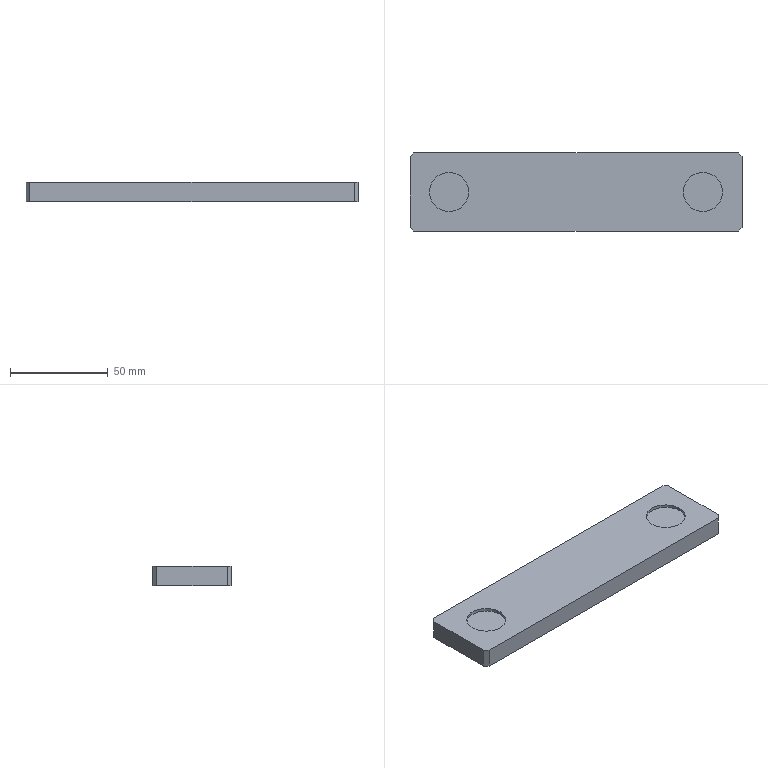Part | SolidWorks | features Chamfer 1, Extrusion 1, ICE 1 | 1 solid | 16 faces | box 170 x 40 x 10 mm | volume 66978 mm3 | plane 12 | cylinder 4 | commonest cylinder face diameters 20 x4
STEP:
#1=CARTESIAN_POINT('',(-75.,0.,8.5));
#2=VERTEX_POINT('',#1);
#3=CARTESIAN_POINT('',(-55.,0.,8.5));
#4=VERTEX_POINT('',#3);
#5=CARTESIAN_POINT('',(-65.,0.,8.5));
#6=DIRECTION('',(0.,0.,1.));
#7=DIRECTION('',(1.,0.,0.));
#8=AXIS2_PLACEMENT_3D('',#5,#6,#7);
#9=CIRCLE('',#8,10.);
#10=EDGE_CURVE('',#2,#4,#9,.T.);
#11=ORIENTED_EDGE('',*,*,#10,.F.);
#12=CARTESIAN_POINT('',(-75.,0.,10.));
#13=VERTEX_POINT('',#12);
#14=CARTESIAN_POINT('',(-75.,0.,8.5));
#15=DIRECTION('',(0.,0.,1.));
#16=VECTOR('',#15,1000.);
#17=LINE('',#14,#16);
#18=EDGE_CURVE('',#2,#13,#17,.T.);
#19=ORIENTED_EDGE('',*,*,#18,.T.);
#20=CARTESIAN_POINT('',(-55.,0.,10.));
#21=VERTEX_POINT('',#20);
#22=CARTESIAN_POINT('',(-65.,0.,10.));
#23=DIRECTION('',(0.,0.,1.));
#24=DIRECTION('',(1.,0.,0.));
#25=AXIS2_PLACEMENT_3D('',#22,#23,#24);
#26=CIRCLE('',#25,10.);
#27=EDGE_CURVE('',#13,#21,#26,.T.);
#28=ORIENTED_EDGE('',*,*,#27,.T.);
#29=CARTESIAN_POINT('',(-55.,0.,8.5));
#30=DIRECTION('',(0.,0.,1.));
#31=VECTOR('',#30,1000.);
#32=LINE('',#29,#31);
#33=EDGE_CURVE('',#4,#21,#32,.T.);
#34=ORIENTED_EDGE('',*,*,#33,.F.);
#35=EDGE_LOOP('',(#11,#19,#28,#34));
#36=FACE_OUTER_BOUND('',#35,.T.);
#37=CARTESIAN_POINT('',(-65.,0.,8.5));
#38=DIRECTION('',(0.,0.,1.));
#39=DIRECTION('',(1.,0.,0.));
#40=AXIS2_PLACEMENT_3D('',#37,#38,#39);
#41=CYLINDRICAL_SURFACE('',#40,10.);
#42=ADVANCED_FACE('',(#36),#41,.F.);
#43=CARTESIAN_POINT('',(55.,0.,8.5));
#44=VERTEX_POINT('',#43);
#45=CARTESIAN_POINT('',(75.,0.,8.5));
#46=VERTEX_POINT('',#45);
#47=CARTESIAN_POINT('',(65.,0.,8.5));
#48=DIRECTION('',(0.,0.,1.));
#49=DIRECTION('',(1.,0.,0.));
#50=AXIS2_PLACEMENT_3D('',#47,#48,#49);
#51=CIRCLE('',#50,10.);
#52=EDGE_CURVE('',#44,#46,#51,.T.);
#53=ORIENTED_EDGE('',*,*,#52,.F.);
#54=CARTESIAN_POINT('',(55.,0.,10.));
#55=VERTEX_POINT('',#54);
#56=CARTESIAN_POINT('',(55.,0.,8.5));
#57=DIRECTION('',(0.,0.,1.));
#58=VECTOR('',#57,1000.);
#59=LINE('',#56,#58);
#60=EDGE_CURVE('',#44,#55,#59,.T.);
#61=ORIENTED_EDGE('',*,*,#60,.T.);
#62=CARTESIAN_POINT('',(75.,0.,10.));
#63=VERTEX_POINT('',#62);
#64=CARTESIAN_POINT('',(65.,0.,10.));
#65=DIRECTION('',(0.,0.,1.));
#66=DIRECTION('',(1.,0.,0.));
#67=AXIS2_PLACEMENT_3D('',#64,#65,#66);
#68=CIRCLE('',#67,10.);
#69=EDGE_CURVE('',#55,#63,#68,.T.);
#70=ORIENTED_EDGE('',*,*,#69,.T.);
#71=CARTESIAN_POINT('',(75.,0.,8.5));
#72=DIRECTION('',(0.,0.,1.));
#73=VECTOR('',#72,1000.);
#74=LINE('',#71,#73);
#75=EDGE_CURVE('',#46,#63,#74,.T.);
#76=ORIENTED_EDGE('',*,*,#75,.F.);
#77=EDGE_LOOP('',(#53,#61,#70,#76));
#78=FACE_OUTER_BOUND('',#77,.T.);
#79=CARTESIAN_POINT('',(65.,0.,8.5));
#80=DIRECTION('',(0.,0.,1.));
#81=DIRECTION('',(1.,0.,0.));
#82=AXIS2_PLACEMENT_3D('',#79,#80,#81);
#83=CYLINDRICAL_SURFACE('',#82,10.);
#84=ADVANCED_FACE('',(#78),#83,.F.);
#85=CARTESIAN_POINT('',(85.,-18.,10.));
#86=VERTEX_POINT('',#85);
#87=CARTESIAN_POINT('',(85.,18.,10.));
#88=VERTEX_POINT('',#87);
#89=CARTESIAN_POINT('',(85.,-20.,10.));
#90=DIRECTION('',(0.,1.,0.));
#91=VECTOR('',#90,1000.);
#92=LINE('',#89,#91);
#93=EDGE_CURVE('',#86,#88,#92,.T.);
#94=ORIENTED_EDGE('',*,*,#93,.F.);
#95=CARTESIAN_POINT('',(85.,-18.,0.));
#96=VERTEX_POINT('',#95);
#97=CARTESIAN_POINT('',(85.,-18.,10.));
#98=DIRECTION('',(0.,0.,-1.));
#99=VECTOR('',#98,1000.);
#100=LINE('',#97,#99);
#101=EDGE_CURVE('',#86,#96,#100,.T.);
#102=ORIENTED_EDGE('',*,*,#101,.T.);
#103=CARTESIAN_POINT('',(85.,18.,0.));
#104=VERTEX_POINT('',#103);
#105=CARTESIAN_POINT('',(85.,-20.,0.));
#106=DIRECTION('',(0.,1.,0.));
#107=VECTOR('',#106,1000.);
#108=LINE('',#105,#107);
#109=EDGE_CURVE('',#96,#104,#108,.T.);
#110=ORIENTED_EDGE('',*,*,#109,.T.);
#111=CARTESIAN_POINT('',(85.,18.,10.));
#112=DIRECTION('',(0.,0.,1.));
#113=VECTOR('',#112,1000.);
#114=LINE('',#111,#113);
#115=EDGE_CURVE('',#104,#88,#114,.T.);
#116=ORIENTED_EDGE('',*,*,#115,.T.);
#117=EDGE_LOOP('',(#94,#102,#110,#116));
#118=FACE_OUTER_BOUND('',#117,.T.);
#119=CARTESIAN_POINT('',(85.,-20.,10.));
#120=DIRECTION('',(-1.,0.,0.));
#121=DIRECTION('',(0.,0.,1.));
#122=AXIS2_PLACEMENT_3D('',#119,#120,#121);
#123=PLANE('',#122);
#124=ADVANCED_FACE('',(#118),#123,.F.);
#125=CARTESIAN_POINT('',(83.,20.,10.));
#126=VERTEX_POINT('',#125);
#127=CARTESIAN_POINT('',(-83.,20.,10.));
#128=VERTEX_POINT('',#127);
#129=CARTESIAN_POINT('',(-85.,20.,10.));
#130=DIRECTION('',(-1.,0.,0.));
#131=VECTOR('',#130,1000.);
#132=LINE('',#129,#131);
#133=EDGE_CURVE('',#126,#128,#132,.T.);
#134=ORIENTED_EDGE('',*,*,#133,.F.);
#135=CARTESIAN_POINT('',(83.,20.,0.));
#136=VERTEX_POINT('',#135);
#137=CARTESIAN_POINT('',(83.,20.,10.));
#138=DIRECTION('',(0.,0.,-1.));
#139=VECTOR('',#138,1000.);
#140=LINE('',#137,#139);
#141=EDGE_CURVE('',#126,#136,#140,.T.);
#142=ORIENTED_EDGE('',*,*,#141,.T.);
#143=CARTESIAN_POINT('',(-83.,20.,0.));
#144=VERTEX_POINT('',#143);
#145=CARTESIAN_POINT('',(-85.,20.,0.));
#146=DIRECTION('',(-1.,0.,0.));
#147=VECTOR('',#146,1000.);
#148=LINE('',#145,#147);
#149=EDGE_CURVE('',#136,#144,#148,.T.);
#150=ORIENTED_EDGE('',*,*,#149,.T.);
#151=CARTESIAN_POINT('',(-83.,20.,10.));
#152=DIRECTION('',(0.,0.,1.));
#153=VECTOR('',#152,1000.);
#154=LINE('',#151,#153);
#155=EDGE_CURVE('',#144,#128,#154,.T.);
#156=ORIENTED_EDGE('',*,*,#155,.T.);
#157=EDGE_LOOP('',(#134,#142,#150,#156));
#158=FACE_OUTER_BOUND('',#157,.T.);
#159=CARTESIAN_POINT('',(-85.,20.,10.));
#160=DIRECTION('',(0.,-1.,0.));
#161=DIRECTION('',(0.,0.,-1.));
#162=AXIS2_PLACEMENT_3D('',#159,#160,#161);
#163=PLANE('',#162);
#164=ADVANCED_FACE('',(#158),#163,.F.);
#165=CARTESIAN_POINT('',(-85.,18.,0.));
#166=VERTEX_POINT('',#165);
#167=CARTESIAN_POINT('',(-85.,-18.,0.));
#168=VERTEX_POINT('',#167);
#169=CARTESIAN_POINT('',(-85.,-20.,0.));
#170=DIRECTION('',(0.,-1.,0.));
#171=VECTOR('',#170,1000.);
#172=LINE('',#169,#171);
#173=EDGE_CURVE('',#166,#168,#172,.T.);
#174=ORIENTED_EDGE('',*,*,#173,.T.);
#175=CARTESIAN_POINT('',(-85.,-18.,10.));
#176=VERTEX_POINT('',#175);
#177=CARTESIAN_POINT('',(-85.,-18.,10.));
#178=DIRECTION('',(0.,0.,1.));
#179=VECTOR('',#178,1000.);
#180=LINE('',#177,#179);
#181=EDGE_CURVE('',#168,#176,#180,.T.);
#182=ORIENTED_EDGE('',*,*,#181,.T.);
#183=CARTESIAN_POINT('',(-85.,18.,10.));
#184=VERTEX_POINT('',#183);
#185=CARTESIAN_POINT('',(-85.,-20.,10.));
#186=DIRECTION('',(0.,-1.,0.));
#187=VECTOR('',#186,1000.);
#188=LINE('',#185,#187);
#189=EDGE_CURVE('',#184,#176,#188,.T.);
#190=ORIENTED_EDGE('',*,*,#189,.F.);
#191=CARTESIAN_POINT('',(-85.,18.,10.));
#192=DIRECTION('',(0.,0.,-1.));
#193=VECTOR('',#192,1000.);
#194=LINE('',#191,#193);
#195=EDGE_CURVE('',#184,#166,#194,.T.);
#196=ORIENTED_EDGE('',*,*,#195,.T.);
#197=EDGE_LOOP('',(#174,#182,#190,#196));
#198=FACE_OUTER_BOUND('',#197,.T.);
#199=CARTESIAN_POINT('',(-85.,-20.,10.));
#200=DIRECTION('',(1.,0.,0.));
#201=DIRECTION('',(0.,0.,-1.));
#202=AXIS2_PLACEMENT_3D('',#199,#200,#201);
#203=PLANE('',#202);
#204=ADVANCED_FACE('',(#198),#203,.F.);
#205=CARTESIAN_POINT('',(-83.,-20.,10.));
#206=VERTEX_POINT('',#205);
#207=CARTESIAN_POINT('',(83.,-20.,10.));
#208=VERTEX_POINT('',#207);
#209=CARTESIAN_POINT('',(-85.,-20.,10.));
#210=DIRECTION('',(1.,0.,0.));
#211=VECTOR('',#210,1000.);
#212=LINE('',#209,#211);
#213=EDGE_CURVE('',#206,#208,#212,.T.);
#214=ORIENTED_EDGE('',*,*,#213,.F.);
#215=CARTESIAN_POINT('',(-83.,-20.,0.));
#216=VERTEX_POINT('',#215);
#217=CARTESIAN_POINT('',(-83.,-20.,10.));
#218=DIRECTION('',(0.,0.,-1.));
#219=VECTOR('',#218,1000.);
#220=LINE('',#217,#219);
#221=EDGE_CURVE('',#206,#216,#220,.T.);
#222=ORIENTED_EDGE('',*,*,#221,.T.);
#223=CARTESIAN_POINT('',(83.,-20.,0.));
#224=VERTEX_POINT('',#223);
#225=CARTESIAN_POINT('',(-85.,-20.,0.));
#226=DIRECTION('',(1.,0.,0.));
#227=VECTOR('',#226,1000.);
#228=LINE('',#225,#227);
#229=EDGE_CURVE('',#216,#224,#228,.T.);
#230=ORIENTED_EDGE('',*,*,#229,.T.);
#231=CARTESIAN_POINT('',(83.,-20.,10.));
#232=DIRECTION('',(0.,0.,1.));
#233=VECTOR('',#232,1000.);
#234=LINE('',#231,#233);
#235=EDGE_CURVE('',#224,#208,#234,.T.);
#236=ORIENTED_EDGE('',*,*,#235,.T.);
#237=EDGE_LOOP('',(#214,#222,#230,#236));
#238=FACE_OUTER_BOUND('',#237,.T.);
#239=CARTESIAN_POINT('',(-85.,-20.,10.));
#240=DIRECTION('',(0.,1.,0.));
#241=DIRECTION('',(0.,0.,1.));
#242=AXIS2_PLACEMENT_3D('',#239,#240,#241);
#243=PLANE('',#242);
#244=ADVANCED_FACE('',(#238),#243,.F.);
#245=CARTESIAN_POINT('',(-65.,0.,10.));
#246=DIRECTION('',(0.,0.,1.));
#247=DIRECTION('',(1.,0.,0.));
#248=AXIS2_PLACEMENT_3D('',#245,#246,#247);
#249=CIRCLE('',#248,10.);
#250=EDGE_CURVE('',#21,#13,#249,.T.);
#251=ORIENTED_EDGE('',*,*,#250,.F.);
#252=ORIENTED_EDGE('',*,*,#27,.F.);
#253=EDGE_LOOP('',(#251,#252));
#254=FACE_BOUND('',#253,.T.);
#255=CARTESIAN_POINT('',(65.,0.,10.));
#256=DIRECTION('',(0.,0.,1.));
#257=DIRECTION('',(1.,0.,0.));
#258=AXIS2_PLACEMENT_3D('',#255,#256,#257);
#259=CIRCLE('',#258,10.);
#260=EDGE_CURVE('',#63,#55,#259,.T.);
#261=ORIENTED_EDGE('',*,*,#260,.F.);
#262=ORIENTED_EDGE('',*,*,#69,.F.);
#263=EDGE_LOOP('',(#261,#262));
#264=FACE_BOUND('',#263,.T.);
#265=ORIENTED_EDGE('',*,*,#189,.T.);
#266=CARTESIAN_POINT('',(-83.,-20.,10.));
#267=DIRECTION('',(0.7071,-0.7071,0.));
#268=VECTOR('',#267,1000.);
#269=LINE('',#266,#268);
#270=EDGE_CURVE('',#176,#206,#269,.T.);
#271=ORIENTED_EDGE('',*,*,#270,.T.);
#272=ORIENTED_EDGE('',*,*,#213,.T.);
#273=CARTESIAN_POINT('',(85.,-18.,10.));
#274=DIRECTION('',(0.7071,0.7071,0.));
#275=VECTOR('',#274,1000.);
#276=LINE('',#273,#275);
#277=EDGE_CURVE('',#208,#86,#276,.T.);
#278=ORIENTED_EDGE('',*,*,#277,.T.);
#279=ORIENTED_EDGE('',*,*,#93,.T.);
#280=CARTESIAN_POINT('',(83.,20.,10.));
#281=DIRECTION('',(-0.7071,0.7071,0.));
#282=VECTOR('',#281,1000.);
#283=LINE('',#280,#282);
#284=EDGE_CURVE('',#88,#126,#283,.T.);
#285=ORIENTED_EDGE('',*,*,#284,.T.);
#286=ORIENTED_EDGE('',*,*,#133,.T.);
#287=CARTESIAN_POINT('',(-85.,18.,10.));
#288=DIRECTION('',(-0.7071,-0.7071,0.));
#289=VECTOR('',#288,1000.);
#290=LINE('',#287,#289);
#291=EDGE_CURVE('',#128,#184,#290,.T.);
#292=ORIENTED_EDGE('',*,*,#291,.T.);
#293=EDGE_LOOP('',(#265,#271,#272,#278,#279,#285,#286,#292));
#294=FACE_OUTER_BOUND('',#293,.T.);
#295=CARTESIAN_POINT('',(0.,0.,10.));
#296=DIRECTION('',(0.,0.,-1.));
#297=DIRECTION('',(-1.,0.,0.));
#298=AXIS2_PLACEMENT_3D('',#295,#296,#297);
#299=PLANE('',#298);
#300=ADVANCED_FACE('',(#254,#264,#294),#299,.F.);
#301=ORIENTED_EDGE('',*,*,#229,.F.);
#302=CARTESIAN_POINT('',(-51.5,-51.5,0.));
#303=DIRECTION('',(-0.7071,0.7071,0.));
#304=VECTOR('',#303,1000.);
#305=LINE('',#302,#304);
#306=EDGE_CURVE('',#216,#168,#305,.T.);
#307=ORIENTED_EDGE('',*,*,#306,.T.);
#308=ORIENTED_EDGE('',*,*,#173,.F.);
#309=CARTESIAN_POINT('',(-51.5,51.5,0.));
#310=DIRECTION('',(0.7071,0.7071,0.));
#311=VECTOR('',#310,1000.);
#312=LINE('',#309,#311);
#313=EDGE_CURVE('',#166,#144,#312,.T.);
#314=ORIENTED_EDGE('',*,*,#313,.T.);
#315=ORIENTED_EDGE('',*,*,#149,.F.);
#316=CARTESIAN_POINT('',(51.5,51.5,0.));
#317=DIRECTION('',(0.7071,-0.7071,0.));
#318=VECTOR('',#317,1000.);
#319=LINE('',#316,#318);
#320=EDGE_CURVE('',#136,#104,#319,.T.);
#321=ORIENTED_EDGE('',*,*,#320,.T.);
#322=ORIENTED_EDGE('',*,*,#109,.F.);
#323=CARTESIAN_POINT('',(51.5,-51.5,0.));
#324=DIRECTION('',(-0.7071,-0.7071,0.));
#325=VECTOR('',#324,1000.);
#326=LINE('',#323,#325);
#327=EDGE_CURVE('',#96,#224,#326,.T.);
#328=ORIENTED_EDGE('',*,*,#327,.T.);
#329=EDGE_LOOP('',(#301,#307,#308,#314,#315,#321,#322,#328));
#330=FACE_OUTER_BOUND('',#329,.T.);
#331=CARTESIAN_POINT('',(0.,0.,0.));
#332=DIRECTION('',(0.,0.,-1.));
#333=DIRECTION('',(-1.,0.,0.));
#334=AXIS2_PLACEMENT_3D('',#331,#332,#333);
#335=PLANE('',#334);
#336=ADVANCED_FACE('',(#330),#335,.T.);
#337=ORIENTED_EDGE('',*,*,#60,.F.);
#338=CARTESIAN_POINT('',(65.,0.,8.5));
#339=DIRECTION('',(0.,0.,1.));
#340=DIRECTION('',(1.,0.,0.));
#341=AXIS2_PLACEMENT_3D('',#338,#339,#340);
#342=CIRCLE('',#341,10.);
#343=EDGE_CURVE('',#46,#44,#342,.T.);
#344=ORIENTED_EDGE('',*,*,#343,.F.);
#345=ORIENTED_EDGE('',*,*,#75,.T.);
#346=ORIENTED_EDGE('',*,*,#260,.T.);
#347=EDGE_LOOP('',(#337,#344,#345,#346));
#348=FACE_OUTER_BOUND('',#347,.T.);
#349=CARTESIAN_POINT('',(65.,0.,8.5));
#350=DIRECTION('',(0.,0.,1.));
#351=DIRECTION('',(1.,0.,0.));
#352=AXIS2_PLACEMENT_3D('',#349,#350,#351);
#353=CYLINDRICAL_SURFACE('',#352,10.);
#354=ADVANCED_FACE('',(#348),#353,.F.);
#355=ORIENTED_EDGE('',*,*,#343,.T.);
#356=ORIENTED_EDGE('',*,*,#52,.T.);
#357=EDGE_LOOP('',(#355,#356));
#358=FACE_OUTER_BOUND('',#357,.T.);
#359=CARTESIAN_POINT('',(65.,0.,8.5));
#360=DIRECTION('',(0.,0.,1.));
#361=DIRECTION('',(1.,0.,0.));
#362=AXIS2_PLACEMENT_3D('',#359,#360,#361);
#363=PLANE('',#362);
#364=ADVANCED_FACE('',(#358),#363,.T.);
#365=ORIENTED_EDGE('',*,*,#18,.F.);
#366=CARTESIAN_POINT('',(-65.,0.,8.5));
#367=DIRECTION('',(0.,0.,1.));
#368=DIRECTION('',(1.,0.,0.));
#369=AXIS2_PLACEMENT_3D('',#366,#367,#368);
#370=CIRCLE('',#369,10.);
#371=EDGE_CURVE('',#4,#2,#370,.T.);
#372=ORIENTED_EDGE('',*,*,#371,.F.);
#373=ORIENTED_EDGE('',*,*,#33,.T.);
#374=ORIENTED_EDGE('',*,*,#250,.T.);
#375=EDGE_LOOP('',(#365,#372,#373,#374));
#376=FACE_OUTER_BOUND('',#375,.T.);
#377=CARTESIAN_POINT('',(-65.,0.,8.5));
#378=DIRECTION('',(0.,0.,1.));
#379=DIRECTION('',(1.,0.,0.));
#380=AXIS2_PLACEMENT_3D('',#377,#378,#379);
#381=CYLINDRICAL_SURFACE('',#380,10.);
#382=ADVANCED_FACE('',(#376),#381,.F.);
#383=ORIENTED_EDGE('',*,*,#371,.T.);
#384=ORIENTED_EDGE('',*,*,#10,.T.);
#385=EDGE_LOOP('',(#383,#384));
#386=FACE_OUTER_BOUND('',#385,.T.);
#387=CARTESIAN_POINT('',(-65.,0.,8.5));
#388=DIRECTION('',(0.,0.,1.));
#389=DIRECTION('',(1.,0.,0.));
#390=AXIS2_PLACEMENT_3D('',#387,#388,#389);
#391=PLANE('',#390);
#392=ADVANCED_FACE('',(#386),#391,.T.);
#393=ORIENTED_EDGE('',*,*,#270,.F.);
#394=ORIENTED_EDGE('',*,*,#181,.F.);
#395=ORIENTED_EDGE('',*,*,#306,.F.);
#396=ORIENTED_EDGE('',*,*,#221,.F.);
#397=EDGE_LOOP('',(#393,#394,#395,#396));
#398=FACE_OUTER_BOUND('',#397,.T.);
#399=CARTESIAN_POINT('',(-83.,-20.,10.));
#400=DIRECTION('',(0.7071,0.7071,0.));
#401=DIRECTION('',(0.,0.,-1.));
#402=AXIS2_PLACEMENT_3D('',#399,#400,#401);
#403=PLANE('',#402);
#404=ADVANCED_FACE('',(#398),#403,.F.);
#405=ORIENTED_EDGE('',*,*,#277,.F.);
#406=ORIENTED_EDGE('',*,*,#235,.F.);
#407=ORIENTED_EDGE('',*,*,#327,.F.);
#408=ORIENTED_EDGE('',*,*,#101,.F.);
#409=EDGE_LOOP('',(#405,#406,#407,#408));
#410=FACE_OUTER_BOUND('',#409,.T.);
#411=CARTESIAN_POINT('',(85.,-18.,10.));
#412=DIRECTION('',(-0.7071,0.7071,0.));
#413=DIRECTION('',(0.,0.,-1.));
#414=AXIS2_PLACEMENT_3D('',#411,#412,#413);
#415=PLANE('',#414);
#416=ADVANCED_FACE('',(#410),#415,.F.);
#417=ORIENTED_EDGE('',*,*,#284,.F.);
#418=ORIENTED_EDGE('',*,*,#115,.F.);
#419=ORIENTED_EDGE('',*,*,#320,.F.);
#420=ORIENTED_EDGE('',*,*,#141,.F.);
#421=EDGE_LOOP('',(#417,#418,#419,#420));
#422=FACE_OUTER_BOUND('',#421,.T.);
#423=CARTESIAN_POINT('',(83.,20.,10.));
#424=DIRECTION('',(-0.7071,-0.7071,0.));
#425=DIRECTION('',(0.,0.,-1.));
#426=AXIS2_PLACEMENT_3D('',#423,#424,#425);
#427=PLANE('',#426);
#428=ADVANCED_FACE('',(#422),#427,.F.);
#429=ORIENTED_EDGE('',*,*,#291,.F.);
#430=ORIENTED_EDGE('',*,*,#155,.F.);
#431=ORIENTED_EDGE('',*,*,#313,.F.);
#432=ORIENTED_EDGE('',*,*,#195,.F.);
#433=EDGE_LOOP('',(#429,#430,#431,#432));
#434=FACE_OUTER_BOUND('',#433,.T.);
#435=CARTESIAN_POINT('',(-85.,18.,10.));
#436=DIRECTION('',(0.7071,-0.7071,0.));
#437=DIRECTION('',(0.,0.,-1.));
#438=AXIS2_PLACEMENT_3D('',#435,#436,#437);
#439=PLANE('',#438);
#440=ADVANCED_FACE('',(#434),#439,.F.);
#441=CLOSED_SHELL('',(#42,#84,#124,#164,#204,#244,#300,#336,#354,#364,#382,#392,#404,#416,#428,#440));
#442=MANIFOLD_SOLID_BREP('',#441);
#443=CARTESIAN_POINT('',(0.,0.,0.));
#444=DIRECTION('',(0.,0.,1.));
#445=DIRECTION('',(1.,0.,0.));
#446=AXIS2_PLACEMENT_3D('',#443,#444,#445);
#447=(LENGTH_UNIT()NAMED_UNIT(*)SI_UNIT(.MILLI.,.METRE.));
#448=UNCERTAINTY_MEASURE_WITH_UNIT(LENGTH_MEASURE(0.00001),#447,'','');
#449=(NAMED_UNIT(*)PLANE_ANGLE_UNIT()SI_UNIT($,.RADIAN.));
#450=(NAMED_UNIT(*)SI_UNIT($,.STERADIAN.)SOLID_ANGLE_UNIT());
#451=(GEOMETRIC_REPRESENTATION_CONTEXT(3)GLOBAL_UNCERTAINTY_ASSIGNED_CONTEXT((#448))GLOBAL_UNIT_ASSIGNED_CONTEXT((#447,#449,#450))REPRESENTATION_CONTEXT('',''));
#452=ADVANCED_BREP_SHAPE_REPRESENTATION('',(#442,#446),#451);